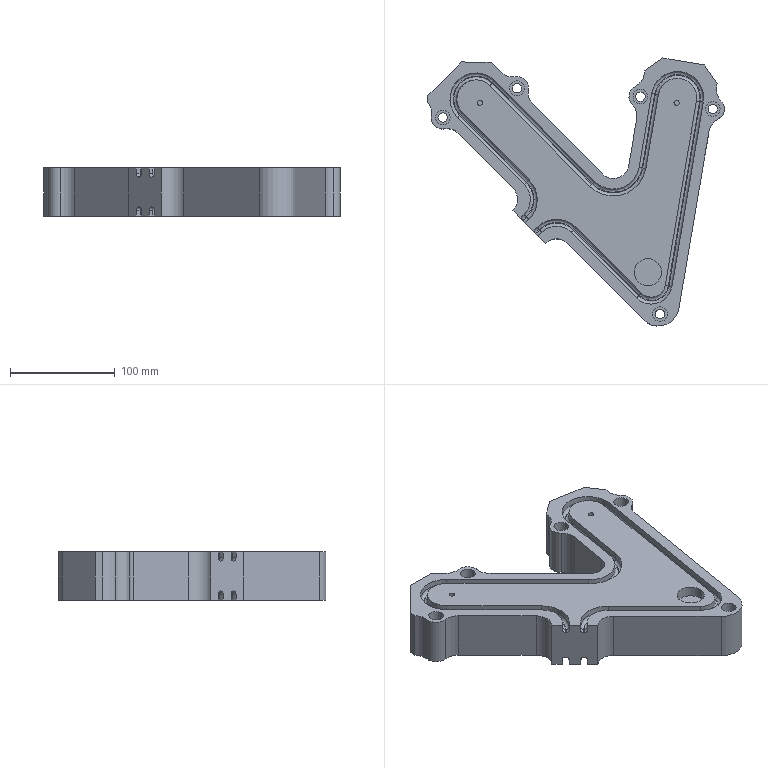Part | Creo | 1 solid | 184 faces | box 282.988 x 255.677 x 46 mm | volume 1446690 mm3 | cylinder 100 | plane 60 | torus 24 | commonest cylinder face diameters 6 x28 30 x11 9 x10 14 x10 5 x8 40 x7